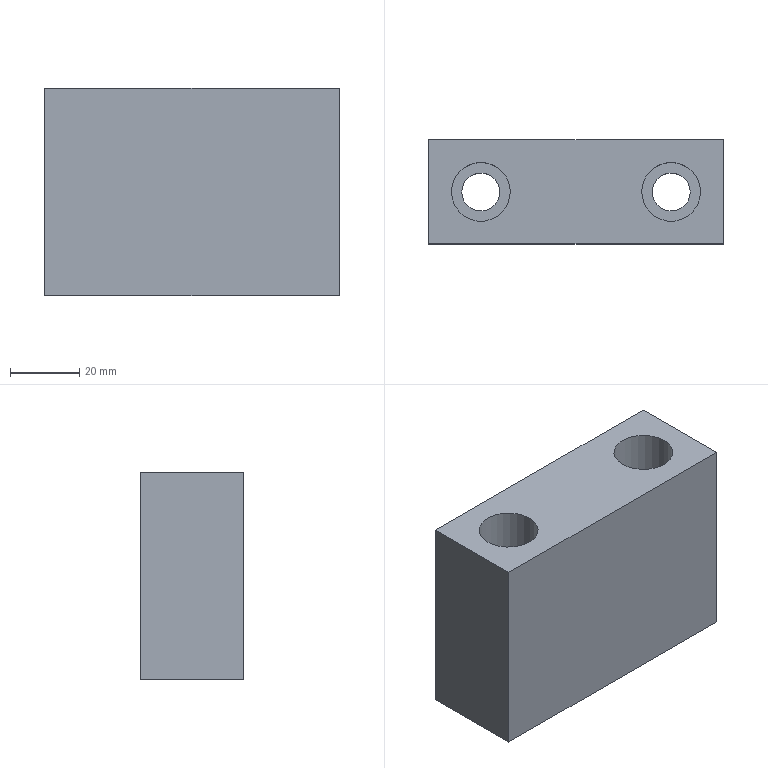Part | STEP file | PN_0002_id1798_x_t | 1 solid | 12 faces | box 85 x 30 x 60 mm | volume 133679 mm3 | plane 8 | cylinder 4 | commonest cylinder face diameters 11 x2 17 x2
STEP:
#1=CARTESIAN_POINT('',(-370.,-262.5,155.));
#2=VERTEX_POINT('',#1);
#3=CARTESIAN_POINT('',(-370.,-262.5,215.));
#4=VERTEX_POINT('',#3);
#5=CARTESIAN_POINT('',(-370.,-262.5,105.));
#6=DIRECTION('',(0.,0.,1.));
#7=VECTOR('',#6,1.);
#8=LINE('',#5,#7);
#9=EDGE_CURVE('',#2,#4,#8,.T.);
#10=ORIENTED_EDGE('',*,*,#9,.F.);
#11=CARTESIAN_POINT('',(-370.,-292.5,155.));
#12=VERTEX_POINT('',#11);
#13=CARTESIAN_POINT('',(-370.,-267.5,155.));
#14=DIRECTION('',(0.,1.,0.));
#15=VECTOR('',#14,1.);
#16=LINE('',#13,#15);
#17=EDGE_CURVE('',#12,#2,#16,.T.);
#18=ORIENTED_EDGE('',*,*,#17,.F.);
#19=CARTESIAN_POINT('',(-370.,-292.5,215.));
#20=VERTEX_POINT('',#19);
#21=CARTESIAN_POINT('',(-370.,-292.5,105.));
#22=DIRECTION('',(0.,0.,1.));
#23=VECTOR('',#22,1.);
#24=LINE('',#21,#23);
#25=EDGE_CURVE('',#12,#20,#24,.T.);
#26=ORIENTED_EDGE('',*,*,#25,.T.);
#27=CARTESIAN_POINT('',(-370.,-267.5,215.));
#28=DIRECTION('',(0.,1.,0.));
#29=VECTOR('',#28,1.);
#30=LINE('',#27,#29);
#31=EDGE_CURVE('',#20,#4,#30,.T.);
#32=ORIENTED_EDGE('',*,*,#31,.T.);
#33=EDGE_LOOP('',(#10,#18,#26,#32));
#34=FACE_OUTER_BOUND('',#33,.T.);
#35=CARTESIAN_POINT('',(-370.,-267.5,105.));
#36=DIRECTION('',(1.,0.,0.));
#37=DIRECTION('',(0.,1.,0.));
#38=AXIS2_PLACEMENT_3D('',#35,#36,#37);
#39=PLANE('',#38);
#40=ADVANCED_FACE('',(#34),#39,.F.);
#41=ORIENTED_EDGE('',*,*,#25,.F.);
#42=CARTESIAN_POINT('',(-285.,-292.5,155.));
#43=VERTEX_POINT('',#42);
#44=CARTESIAN_POINT('',(-327.5,-292.5,155.));
#45=DIRECTION('',(-1.,0.,0.));
#46=VECTOR('',#45,1.);
#47=LINE('',#44,#46);
#48=EDGE_CURVE('',#43,#12,#47,.T.);
#49=ORIENTED_EDGE('',*,*,#48,.F.);
#50=CARTESIAN_POINT('',(-285.,-292.5,215.));
#51=VERTEX_POINT('',#50);
#52=CARTESIAN_POINT('',(-285.,-292.5,105.));
#53=DIRECTION('',(0.,0.,1.));
#54=VECTOR('',#53,1.);
#55=LINE('',#52,#54);
#56=EDGE_CURVE('',#43,#51,#55,.T.);
#57=ORIENTED_EDGE('',*,*,#56,.T.);
#58=CARTESIAN_POINT('',(-327.5,-292.5,215.));
#59=DIRECTION('',(-1.,0.,0.));
#60=VECTOR('',#59,1.);
#61=LINE('',#58,#60);
#62=EDGE_CURVE('',#51,#20,#61,.T.);
#63=ORIENTED_EDGE('',*,*,#62,.T.);
#64=EDGE_LOOP('',(#41,#49,#57,#63));
#65=FACE_OUTER_BOUND('',#64,.T.);
#66=CARTESIAN_POINT('',(-327.5,-292.5,105.));
#67=DIRECTION('',(0.,1.,0.));
#68=DIRECTION('',(-1.,0.,0.));
#69=AXIS2_PLACEMENT_3D('',#66,#67,#68);
#70=PLANE('',#69);
#71=ADVANCED_FACE('',(#65),#70,.F.);
#72=ORIENTED_EDGE('',*,*,#56,.F.);
#73=CARTESIAN_POINT('',(-285.,-262.5,155.));
#74=VERTEX_POINT('',#73);
#75=CARTESIAN_POINT('',(-285.,-267.5,155.));
#76=DIRECTION('',(0.,-1.,0.));
#77=VECTOR('',#76,1.);
#78=LINE('',#75,#77);
#79=EDGE_CURVE('',#74,#43,#78,.T.);
#80=ORIENTED_EDGE('',*,*,#79,.F.);
#81=CARTESIAN_POINT('',(-285.,-262.5,215.));
#82=VERTEX_POINT('',#81);
#83=CARTESIAN_POINT('',(-285.,-262.5,105.));
#84=DIRECTION('',(0.,0.,1.));
#85=VECTOR('',#84,1.);
#86=LINE('',#83,#85);
#87=EDGE_CURVE('',#74,#82,#86,.T.);
#88=ORIENTED_EDGE('',*,*,#87,.T.);
#89=CARTESIAN_POINT('',(-285.,-267.5,215.));
#90=DIRECTION('',(0.,-1.,0.));
#91=VECTOR('',#90,1.);
#92=LINE('',#89,#91);
#93=EDGE_CURVE('',#82,#51,#92,.T.);
#94=ORIENTED_EDGE('',*,*,#93,.T.);
#95=EDGE_LOOP('',(#72,#80,#88,#94));
#96=FACE_OUTER_BOUND('',#95,.T.);
#97=CARTESIAN_POINT('',(-285.,-267.5,105.));
#98=DIRECTION('',(-1.,0.,0.));
#99=DIRECTION('',(0.,-1.,0.));
#100=AXIS2_PLACEMENT_3D('',#97,#98,#99);
#101=PLANE('',#100);
#102=ADVANCED_FACE('',(#96),#101,.F.);
#103=CARTESIAN_POINT('',(-327.5,-262.5,155.));
#104=DIRECTION('',(1.,0.,0.));
#105=VECTOR('',#104,1.);
#106=LINE('',#103,#105);
#107=EDGE_CURVE('',#2,#74,#106,.T.);
#108=ORIENTED_EDGE('',*,*,#107,.F.);
#109=ORIENTED_EDGE('',*,*,#9,.T.);
#110=CARTESIAN_POINT('',(-327.5,-262.5,215.));
#111=DIRECTION('',(1.,0.,0.));
#112=VECTOR('',#111,1.);
#113=LINE('',#110,#112);
#114=EDGE_CURVE('',#4,#82,#113,.T.);
#115=ORIENTED_EDGE('',*,*,#114,.T.);
#116=ORIENTED_EDGE('',*,*,#87,.F.);
#117=EDGE_LOOP('',(#108,#109,#115,#116));
#118=FACE_OUTER_BOUND('',#117,.T.);
#119=CARTESIAN_POINT('',(-327.5,-262.5,105.));
#120=DIRECTION('',(0.,1.,0.));
#121=DIRECTION('',(-1.,0.,0.));
#122=AXIS2_PLACEMENT_3D('',#119,#120,#121);
#123=PLANE('',#122);
#124=ADVANCED_FACE('',(#118),#123,.T.);
#125=CARTESIAN_POINT('',(-291.5,-277.5,215.));
#126=VERTEX_POINT('',#125);
#127=CARTESIAN_POINT('',(-300.,-277.5,215.));
#128=DIRECTION('',(0.,0.,1.));
#129=DIRECTION('',(1.,0.,0.));
#130=AXIS2_PLACEMENT_3D('',#127,#128,#129);
#131=CIRCLE('',#130,8.5);
#132=EDGE_CURVE('',#126,#126,#131,.T.);
#133=ORIENTED_EDGE('',*,*,#132,.F.);
#134=EDGE_LOOP('',(#133));
#135=FACE_BOUND('',#134,.T.);
#136=CARTESIAN_POINT('',(-363.5,-277.5,215.));
#137=VERTEX_POINT('',#136);
#138=CARTESIAN_POINT('',(-355.,-277.5,215.));
#139=DIRECTION('',(0.,0.,-1.));
#140=DIRECTION('',(-1.,0.,0.));
#141=AXIS2_PLACEMENT_3D('',#138,#139,#140);
#142=CIRCLE('',#141,8.5);
#143=EDGE_CURVE('',#137,#137,#142,.T.);
#144=ORIENTED_EDGE('',*,*,#143,.T.);
#145=EDGE_LOOP('',(#144));
#146=FACE_BOUND('',#145,.T.);
#147=ORIENTED_EDGE('',*,*,#93,.F.);
#148=ORIENTED_EDGE('',*,*,#114,.F.);
#149=ORIENTED_EDGE('',*,*,#31,.F.);
#150=ORIENTED_EDGE('',*,*,#62,.F.);
#151=EDGE_LOOP('',(#147,#148,#149,#150));
#152=FACE_BOUND('',#151,.T.);
#153=CARTESIAN_POINT('',(253.5,-1.,215.));
#154=DIRECTION('',(0.,0.,-1.));
#155=DIRECTION('',(1.,0.,0.));
#156=AXIS2_PLACEMENT_3D('',#153,#154,#155);
#157=PLANE('',#156);
#158=ADVANCED_FACE('',(#135,#146,#152),#157,.F.);
#159=CARTESIAN_POINT('',(-305.5,-277.5,155.));
#160=VERTEX_POINT('',#159);
#161=CARTESIAN_POINT('',(-300.,-277.5,155.));
#162=DIRECTION('',(0.,0.,-1.));
#163=DIRECTION('',(-1.,0.,0.));
#164=AXIS2_PLACEMENT_3D('',#161,#162,#163);
#165=CIRCLE('',#164,5.5);
#166=EDGE_CURVE('',#160,#160,#165,.T.);
#167=ORIENTED_EDGE('',*,*,#166,.F.);
#168=EDGE_LOOP('',(#167));
#169=FACE_BOUND('',#168,.T.);
#170=CARTESIAN_POINT('',(-349.5,-277.5,155.));
#171=VERTEX_POINT('',#170);
#172=CARTESIAN_POINT('',(-355.,-277.5,155.));
#173=DIRECTION('',(0.,0.,1.));
#174=DIRECTION('',(1.,0.,0.));
#175=AXIS2_PLACEMENT_3D('',#172,#173,#174);
#176=CIRCLE('',#175,5.5);
#177=EDGE_CURVE('',#171,#171,#176,.T.);
#178=ORIENTED_EDGE('',*,*,#177,.T.);
#179=EDGE_LOOP('',(#178));
#180=FACE_BOUND('',#179,.T.);
#181=ORIENTED_EDGE('',*,*,#79,.T.);
#182=ORIENTED_EDGE('',*,*,#48,.T.);
#183=ORIENTED_EDGE('',*,*,#17,.T.);
#184=ORIENTED_EDGE('',*,*,#107,.T.);
#185=EDGE_LOOP('',(#181,#182,#183,#184));
#186=FACE_BOUND('',#185,.T.);
#187=CARTESIAN_POINT('',(253.5,-1.,155.));
#188=DIRECTION('',(0.,0.,-1.));
#189=DIRECTION('',(1.,0.,0.));
#190=AXIS2_PLACEMENT_3D('',#187,#188,#189);
#191=PLANE('',#190);
#192=ADVANCED_FACE('',(#169,#180,#186),#191,.T.);
#193=CARTESIAN_POINT('',(-360.5,-277.5,185.));
#194=VERTEX_POINT('',#193);
#195=CARTESIAN_POINT('',(-355.,-277.5,185.));
#196=DIRECTION('',(0.,0.,-1.));
#197=DIRECTION('',(-1.,0.,0.));
#198=AXIS2_PLACEMENT_3D('',#195,#196,#197);
#199=CIRCLE('',#198,5.5);
#200=EDGE_CURVE('',#194,#194,#199,.T.);
#201=ORIENTED_EDGE('',*,*,#200,.F.);
#202=EDGE_LOOP('',(#201));
#203=FACE_BOUND('',#202,.T.);
#204=ORIENTED_EDGE('',*,*,#177,.F.);
#205=EDGE_LOOP('',(#204));
#206=FACE_BOUND('',#205,.T.);
#207=CARTESIAN_POINT('',(-355.,-277.5,155.));
#208=DIRECTION('',(0.,0.,1.));
#209=DIRECTION('',(1.,0.,0.));
#210=AXIS2_PLACEMENT_3D('',#207,#208,#209);
#211=CYLINDRICAL_SURFACE('',#210,5.5);
#212=ADVANCED_FACE('',(#203,#206),#211,.F.);
#213=ORIENTED_EDGE('',*,*,#200,.T.);
#214=EDGE_LOOP('',(#213));
#215=FACE_BOUND('',#214,.T.);
#216=CARTESIAN_POINT('',(-346.5,-277.5,185.));
#217=VERTEX_POINT('',#216);
#218=CARTESIAN_POINT('',(-355.,-277.5,185.));
#219=DIRECTION('',(0.,0.,-1.));
#220=DIRECTION('',(1.,0.,0.));
#221=AXIS2_PLACEMENT_3D('',#218,#219,#220);
#222=CIRCLE('',#221,8.5);
#223=EDGE_CURVE('',#217,#217,#222,.T.);
#224=ORIENTED_EDGE('',*,*,#223,.F.);
#225=EDGE_LOOP('',(#224));
#226=FACE_BOUND('',#225,.T.);
#227=CARTESIAN_POINT('',(-355.,-277.5,185.));
#228=DIRECTION('',(0.,0.,-1.));
#229=DIRECTION('',(-1.,0.,0.));
#230=AXIS2_PLACEMENT_3D('',#227,#228,#229);
#231=PLANE('',#230);
#232=ADVANCED_FACE('',(#215,#226),#231,.F.);
#233=ORIENTED_EDGE('',*,*,#143,.F.);
#234=EDGE_LOOP('',(#233));
#235=FACE_BOUND('',#234,.T.);
#236=ORIENTED_EDGE('',*,*,#223,.T.);
#237=EDGE_LOOP('',(#236));
#238=FACE_BOUND('',#237,.T.);
#239=CARTESIAN_POINT('',(-355.,-277.5,185.));
#240=DIRECTION('',(0.,0.,1.));
#241=DIRECTION('',(1.,0.,0.));
#242=AXIS2_PLACEMENT_3D('',#239,#240,#241);
#243=CYLINDRICAL_SURFACE('',#242,8.5);
#244=ADVANCED_FACE('',(#235,#238),#243,.F.);
#245=CARTESIAN_POINT('',(-294.5,-277.5,185.));
#246=VERTEX_POINT('',#245);
#247=CARTESIAN_POINT('',(-300.,-277.5,185.));
#248=DIRECTION('',(0.,0.,1.));
#249=DIRECTION('',(1.,0.,0.));
#250=AXIS2_PLACEMENT_3D('',#247,#248,#249);
#251=CIRCLE('',#250,5.5);
#252=EDGE_CURVE('',#246,#246,#251,.T.);
#253=ORIENTED_EDGE('',*,*,#252,.T.);
#254=EDGE_LOOP('',(#253));
#255=FACE_BOUND('',#254,.T.);
#256=ORIENTED_EDGE('',*,*,#166,.T.);
#257=EDGE_LOOP('',(#256));
#258=FACE_BOUND('',#257,.T.);
#259=CARTESIAN_POINT('',(-300.,-277.5,155.));
#260=DIRECTION('',(0.,0.,1.));
#261=DIRECTION('',(-1.,0.,0.));
#262=AXIS2_PLACEMENT_3D('',#259,#260,#261);
#263=CYLINDRICAL_SURFACE('',#262,5.5);
#264=ADVANCED_FACE('',(#255,#258),#263,.F.);
#265=ORIENTED_EDGE('',*,*,#252,.F.);
#266=EDGE_LOOP('',(#265));
#267=FACE_BOUND('',#266,.T.);
#268=CARTESIAN_POINT('',(-308.5,-277.5,185.));
#269=VERTEX_POINT('',#268);
#270=CARTESIAN_POINT('',(-300.,-277.5,185.));
#271=DIRECTION('',(0.,0.,1.));
#272=DIRECTION('',(-1.,0.,0.));
#273=AXIS2_PLACEMENT_3D('',#270,#271,#272);
#274=CIRCLE('',#273,8.5);
#275=EDGE_CURVE('',#269,#269,#274,.T.);
#276=ORIENTED_EDGE('',*,*,#275,.T.);
#277=EDGE_LOOP('',(#276));
#278=FACE_BOUND('',#277,.T.);
#279=CARTESIAN_POINT('',(-300.,-277.5,185.));
#280=DIRECTION('',(0.,0.,-1.));
#281=DIRECTION('',(1.,0.,0.));
#282=AXIS2_PLACEMENT_3D('',#279,#280,#281);
#283=PLANE('',#282);
#284=ADVANCED_FACE('',(#267,#278),#283,.F.);
#285=ORIENTED_EDGE('',*,*,#132,.T.);
#286=EDGE_LOOP('',(#285));
#287=FACE_BOUND('',#286,.T.);
#288=ORIENTED_EDGE('',*,*,#275,.F.);
#289=EDGE_LOOP('',(#288));
#290=FACE_BOUND('',#289,.T.);
#291=CARTESIAN_POINT('',(-300.,-277.5,185.));
#292=DIRECTION('',(0.,0.,1.));
#293=DIRECTION('',(-1.,0.,0.));
#294=AXIS2_PLACEMENT_3D('',#291,#292,#293);
#295=CYLINDRICAL_SURFACE('',#294,8.5);
#296=ADVANCED_FACE('',(#287,#290),#295,.F.);
#297=CLOSED_SHELL('',(#40,#71,#102,#124,#158,#192,#212,#232,#244,#264,#284,#296));
#298=MANIFOLD_SOLID_BREP('',#297);
#299=(LENGTH_UNIT()NAMED_UNIT(*)SI_UNIT(.MILLI.,.METRE.));
#300=UNCERTAINTY_MEASURE_WITH_UNIT(LENGTH_MEASURE(0.00002),#299,'','');
#301=(NAMED_UNIT(*)PLANE_ANGLE_UNIT()SI_UNIT($,.RADIAN.));
#302=PLANE_ANGLE_MEASURE_WITH_UNIT(PLANE_ANGLE_MEASURE(0.01745),#301);
#303=DIMENSIONAL_EXPONENTS(0.,0.,0.,0.,0.,0.,0.);
#304=(CONVERSION_BASED_UNIT('DEGREE',#302)NAMED_UNIT(#303)PLANE_ANGLE_UNIT());
#305=(NAMED_UNIT(*)SI_UNIT($,.STERADIAN.)SOLID_ANGLE_UNIT());
#306=(GEOMETRIC_REPRESENTATION_CONTEXT(3)GLOBAL_UNCERTAINTY_ASSIGNED_CONTEXT((#300))GLOBAL_UNIT_ASSIGNED_CONTEXT((#299,#304,#305))REPRESENTATION_CONTEXT('',''));
#307=ADVANCED_BREP_SHAPE_REPRESENTATION('',(#298),#306);